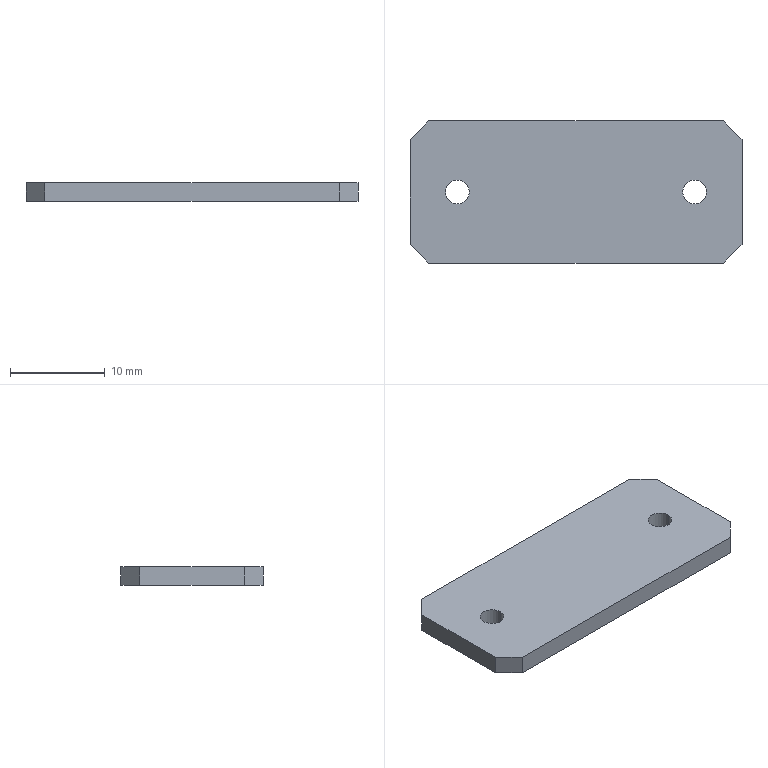Part | STEP file | 227H056374 Sensor Dog_Default | 1 solid | 14 faces | box 35 x 15 x 2 mm | volume 1014 mm3 | plane 10 | cylinder 4 | commonest cylinder face diameters 2.5 x4
STEP:
#1=CARTESIAN_POINT('',(0.,0.,0.));
#2=DIRECTION('',(0.,0.,1.));
#3=DIRECTION('',(1.,0.,0.));
#4=AXIS2_PLACEMENT_3D('',#1,#2,#3);
#5=CARTESIAN_POINT('',(-6.25,7.5,0.));
#6=VERTEX_POINT('',#5);
#7=CARTESIAN_POINT('',(-6.25,7.5,-2.));
#8=VERTEX_POINT('',#7);
#9=CARTESIAN_POINT('',(-6.25,7.5,-2.));
#10=DIRECTION('',(0.,0.,-1.));
#11=VECTOR('',#10,1.);
#12=LINE('',#9,#11);
#13=CARTESIAN_POINT('',(-5.,7.5,-2.));
#14=DIRECTION('',(0.,0.,-1.));
#15=DIRECTION('',(-1.,0.,0.));
#16=AXIS2_PLACEMENT_3D('',#13,#14,#15);
#17=CYLINDRICAL_SURFACE('',#16,1.25);
#18=CARTESIAN_POINT('',(6.283,0.));
#19=DIRECTION('',(0.,1.));
#20=VECTOR('',#19,1.);
#21=LINE('',#18,#20);
#22=(GEOMETRIC_REPRESENTATION_CONTEXT(2)PARAMETRIC_REPRESENTATION_CONTEXT()REPRESENTATION_CONTEXT('',''));
#23=DEFINITIONAL_REPRESENTATION('',(#21),#22);
#24=PCURVE('',#17,#23);
#25=CARTESIAN_POINT('',(-5.,7.5,-2.));
#26=DIRECTION('',(0.,0.,-1.));
#27=DIRECTION('',(-1.,0.,0.));
#28=AXIS2_PLACEMENT_3D('',#25,#26,#27);
#29=CYLINDRICAL_SURFACE('',#28,1.25);
#30=CARTESIAN_POINT('',(0.,0.));
#31=DIRECTION('',(0.,1.));
#32=VECTOR('',#31,1.);
#33=LINE('',#30,#32);
#34=(GEOMETRIC_REPRESENTATION_CONTEXT(2)PARAMETRIC_REPRESENTATION_CONTEXT()REPRESENTATION_CONTEXT('',''));
#35=DEFINITIONAL_REPRESENTATION('',(#33),#34);
#36=PCURVE('',#29,#35);
#37=SURFACE_CURVE('',#12,(#24,#36),.PCURVE_S1.);
#38=EDGE_CURVE('',#6,#8,#37,.T.);
#39=ORIENTED_EDGE('',*,*,#38,.T.);
#40=CARTESIAN_POINT('',(-3.75,7.5,-2.));
#41=VERTEX_POINT('',#40);
#42=CARTESIAN_POINT('',(-5.,7.5,-2.));
#43=DIRECTION('',(0.,0.,-1.));
#44=DIRECTION('',(-1.,0.,0.));
#45=AXIS2_PLACEMENT_3D('',#42,#43,#44);
#46=CIRCLE('',#45,1.25);
#47=CARTESIAN_POINT('',(0.,0.));
#48=DIRECTION('',(1.,0.));
#49=VECTOR('',#48,1.);
#50=LINE('',#47,#49);
#51=(GEOMETRIC_REPRESENTATION_CONTEXT(2)PARAMETRIC_REPRESENTATION_CONTEXT()REPRESENTATION_CONTEXT('',''));
#52=DEFINITIONAL_REPRESENTATION('',(#50),#51);
#53=PCURVE('',#17,#52);
#54=CARTESIAN_POINT('',(0.,15.,-2.));
#55=DIRECTION('',(0.,0.,1.));
#56=DIRECTION('',(1.,0.,0.));
#57=AXIS2_PLACEMENT_3D('',#54,#55,#56);
#58=PLANE('',#57);
#59=CARTESIAN_POINT('',(-6.25,-7.5));
#60=CARTESIAN_POINT('',(-6.25,-5.335));
#61=CARTESIAN_POINT('',(-4.375,-6.417));
#62=CARTESIAN_POINT('',(-2.5,-7.5));
#63=CARTESIAN_POINT('',(-4.375,-8.583));
#64=CARTESIAN_POINT('',(-6.25,-9.665));
#65=CARTESIAN_POINT('',(-6.25,-7.5));
#66=(BOUNDED_CURVE()B_SPLINE_CURVE(2,(#59,#60,#61,#62,#63,#64,#65),.UNSPECIFIED.,.T.,.F.)B_SPLINE_CURVE_WITH_KNOTS((1,2,2,2,2,1),(-2.094,0.,2.094,4.189,6.283,8.378),.UNSPECIFIED.)CURVE()GEOMETRIC_REPRESENTATION_ITEM()RATIONAL_B_SPLINE_CURVE((1.,0.5,1.,0.5,1.,0.5,1.))REPRESENTATION_ITEM(''));
#67=(GEOMETRIC_REPRESENTATION_CONTEXT(2)PARAMETRIC_REPRESENTATION_CONTEXT()REPRESENTATION_CONTEXT('',''));
#68=DEFINITIONAL_REPRESENTATION('',(#66),#67);
#69=PCURVE('',#58,#68);
#70=SURFACE_CURVE('',#46,(#53,#69),.PCURVE_S1.);
#71=EDGE_CURVE('',#41,#8,#70,.T.);
#72=ORIENTED_EDGE('',*,*,#71,.F.);
#73=CARTESIAN_POINT('',(-3.75,7.5,0.));
#74=VERTEX_POINT('',#73);
#75=CARTESIAN_POINT('',(-3.75,7.5,-2.));
#76=DIRECTION('',(0.,0.,-1.));
#77=VECTOR('',#76,1.);
#78=LINE('',#75,#77);
#79=CARTESIAN_POINT('',(3.142,0.));
#80=DIRECTION('',(0.,1.));
#81=VECTOR('',#80,1.);
#82=LINE('',#79,#81);
#83=(GEOMETRIC_REPRESENTATION_CONTEXT(2)PARAMETRIC_REPRESENTATION_CONTEXT()REPRESENTATION_CONTEXT('',''));
#84=DEFINITIONAL_REPRESENTATION('',(#82),#83);
#85=PCURVE('',#17,#84);
#86=CARTESIAN_POINT('',(3.142,0.));
#87=DIRECTION('',(0.,1.));
#88=VECTOR('',#87,1.);
#89=LINE('',#86,#88);
#90=(GEOMETRIC_REPRESENTATION_CONTEXT(2)PARAMETRIC_REPRESENTATION_CONTEXT()REPRESENTATION_CONTEXT('',''));
#91=DEFINITIONAL_REPRESENTATION('',(#89),#90);
#92=PCURVE('',#29,#91);
#93=SURFACE_CURVE('',#78,(#85,#92),.PCURVE_S1.);
#94=EDGE_CURVE('',#74,#41,#93,.T.);
#95=ORIENTED_EDGE('',*,*,#94,.F.);
#96=CARTESIAN_POINT('',(-5.,7.5,0.));
#97=DIRECTION('',(0.,0.,1.));
#98=DIRECTION('',(1.,0.,0.));
#99=AXIS2_PLACEMENT_3D('',#96,#97,#98);
#100=CIRCLE('',#99,1.25);
#101=CARTESIAN_POINT('',(9.425,-2.));
#102=DIRECTION('',(-1.,0.));
#103=VECTOR('',#102,1.);
#104=LINE('',#101,#103);
#105=(GEOMETRIC_REPRESENTATION_CONTEXT(2)PARAMETRIC_REPRESENTATION_CONTEXT()REPRESENTATION_CONTEXT('',''));
#106=DEFINITIONAL_REPRESENTATION('',(#104),#105);
#107=PCURVE('',#17,#106);
#108=CARTESIAN_POINT('',(0.,15.,0.));
#109=DIRECTION('',(0.,0.,1.));
#110=DIRECTION('',(1.,0.,0.));
#111=AXIS2_PLACEMENT_3D('',#108,#109,#110);
#112=PLANE('',#111);
#113=CARTESIAN_POINT('',(-5.,-7.5));
#114=DIRECTION('',(1.,0.));
#115=AXIS2_PLACEMENT_2D('',#113,#114);
#116=CIRCLE('',#115,1.25);
#117=(GEOMETRIC_REPRESENTATION_CONTEXT(2)PARAMETRIC_REPRESENTATION_CONTEXT()REPRESENTATION_CONTEXT('',''));
#118=DEFINITIONAL_REPRESENTATION('',(#116),#117);
#119=PCURVE('',#112,#118);
#120=SURFACE_CURVE('',#100,(#107,#119),.PCURVE_S1.);
#121=EDGE_CURVE('',#6,#74,#120,.T.);
#122=ORIENTED_EDGE('',*,*,#121,.F.);
#123=EDGE_LOOP('',(#39,#72,#95,#122));
#124=FACE_BOUND('',#123,.F.);
#125=ADVANCED_FACE('',(#124),#17,.F.);
#126=CARTESIAN_POINT('',(-31.25,7.5,0.));
#127=VERTEX_POINT('',#126);
#128=CARTESIAN_POINT('',(-31.25,7.5,-2.));
#129=VERTEX_POINT('',#128);
#130=CARTESIAN_POINT('',(-31.25,7.5,-2.));
#131=DIRECTION('',(0.,0.,-1.));
#132=VECTOR('',#131,1.);
#133=LINE('',#130,#132);
#134=CARTESIAN_POINT('',(-30.,7.5,-2.));
#135=DIRECTION('',(0.,0.,-1.));
#136=DIRECTION('',(-1.,0.,0.));
#137=AXIS2_PLACEMENT_3D('',#134,#135,#136);
#138=CYLINDRICAL_SURFACE('',#137,1.25);
#139=CARTESIAN_POINT('',(6.283,0.));
#140=DIRECTION('',(0.,1.));
#141=VECTOR('',#140,1.);
#142=LINE('',#139,#141);
#143=(GEOMETRIC_REPRESENTATION_CONTEXT(2)PARAMETRIC_REPRESENTATION_CONTEXT()REPRESENTATION_CONTEXT('',''));
#144=DEFINITIONAL_REPRESENTATION('',(#142),#143);
#145=PCURVE('',#138,#144);
#146=CARTESIAN_POINT('',(-30.,7.5,-2.));
#147=DIRECTION('',(0.,0.,-1.));
#148=DIRECTION('',(-1.,0.,0.));
#149=AXIS2_PLACEMENT_3D('',#146,#147,#148);
#150=CYLINDRICAL_SURFACE('',#149,1.25);
#151=CARTESIAN_POINT('',(0.,0.));
#152=DIRECTION('',(0.,1.));
#153=VECTOR('',#152,1.);
#154=LINE('',#151,#153);
#155=(GEOMETRIC_REPRESENTATION_CONTEXT(2)PARAMETRIC_REPRESENTATION_CONTEXT()REPRESENTATION_CONTEXT('',''));
#156=DEFINITIONAL_REPRESENTATION('',(#154),#155);
#157=PCURVE('',#150,#156);
#158=SURFACE_CURVE('',#133,(#145,#157),.PCURVE_S1.);
#159=EDGE_CURVE('',#127,#129,#158,.T.);
#160=ORIENTED_EDGE('',*,*,#159,.T.);
#161=CARTESIAN_POINT('',(-28.75,7.5,-2.));
#162=VERTEX_POINT('',#161);
#163=CARTESIAN_POINT('',(-30.,7.5,-2.));
#164=DIRECTION('',(0.,0.,-1.));
#165=DIRECTION('',(-1.,0.,0.));
#166=AXIS2_PLACEMENT_3D('',#163,#164,#165);
#167=CIRCLE('',#166,1.25);
#168=CARTESIAN_POINT('',(0.,0.));
#169=DIRECTION('',(1.,0.));
#170=VECTOR('',#169,1.);
#171=LINE('',#168,#170);
#172=(GEOMETRIC_REPRESENTATION_CONTEXT(2)PARAMETRIC_REPRESENTATION_CONTEXT()REPRESENTATION_CONTEXT('',''));
#173=DEFINITIONAL_REPRESENTATION('',(#171),#172);
#174=PCURVE('',#138,#173);
#175=CARTESIAN_POINT('',(-31.25,-7.5));
#176=CARTESIAN_POINT('',(-31.25,-5.335));
#177=CARTESIAN_POINT('',(-29.375,-6.417));
#178=CARTESIAN_POINT('',(-27.5,-7.5));
#179=CARTESIAN_POINT('',(-29.375,-8.583));
#180=CARTESIAN_POINT('',(-31.25,-9.665));
#181=CARTESIAN_POINT('',(-31.25,-7.5));
#182=(BOUNDED_CURVE()B_SPLINE_CURVE(2,(#175,#176,#177,#178,#179,#180,#181),.UNSPECIFIED.,.T.,.F.)B_SPLINE_CURVE_WITH_KNOTS((1,2,2,2,2,1),(-2.094,0.,2.094,4.189,6.283,8.378),.UNSPECIFIED.)CURVE()GEOMETRIC_REPRESENTATION_ITEM()RATIONAL_B_SPLINE_CURVE((1.,0.5,1.,0.5,1.,0.5,1.))REPRESENTATION_ITEM(''));
#183=(GEOMETRIC_REPRESENTATION_CONTEXT(2)PARAMETRIC_REPRESENTATION_CONTEXT()REPRESENTATION_CONTEXT('',''));
#184=DEFINITIONAL_REPRESENTATION('',(#182),#183);
#185=PCURVE('',#58,#184);
#186=SURFACE_CURVE('',#167,(#174,#185),.PCURVE_S1.);
#187=EDGE_CURVE('',#162,#129,#186,.T.);
#188=ORIENTED_EDGE('',*,*,#187,.F.);
#189=CARTESIAN_POINT('',(-28.75,7.5,0.));
#190=VERTEX_POINT('',#189);
#191=CARTESIAN_POINT('',(-28.75,7.5,-2.));
#192=DIRECTION('',(0.,0.,-1.));
#193=VECTOR('',#192,1.);
#194=LINE('',#191,#193);
#195=CARTESIAN_POINT('',(3.142,0.));
#196=DIRECTION('',(0.,1.));
#197=VECTOR('',#196,1.);
#198=LINE('',#195,#197);
#199=(GEOMETRIC_REPRESENTATION_CONTEXT(2)PARAMETRIC_REPRESENTATION_CONTEXT()REPRESENTATION_CONTEXT('',''));
#200=DEFINITIONAL_REPRESENTATION('',(#198),#199);
#201=PCURVE('',#138,#200);
#202=CARTESIAN_POINT('',(3.142,0.));
#203=DIRECTION('',(0.,1.));
#204=VECTOR('',#203,1.);
#205=LINE('',#202,#204);
#206=(GEOMETRIC_REPRESENTATION_CONTEXT(2)PARAMETRIC_REPRESENTATION_CONTEXT()REPRESENTATION_CONTEXT('',''));
#207=DEFINITIONAL_REPRESENTATION('',(#205),#206);
#208=PCURVE('',#150,#207);
#209=SURFACE_CURVE('',#194,(#201,#208),.PCURVE_S1.);
#210=EDGE_CURVE('',#190,#162,#209,.T.);
#211=ORIENTED_EDGE('',*,*,#210,.F.);
#212=CARTESIAN_POINT('',(-30.,7.5,0.));
#213=DIRECTION('',(0.,0.,1.));
#214=DIRECTION('',(1.,0.,0.));
#215=AXIS2_PLACEMENT_3D('',#212,#213,#214);
#216=CIRCLE('',#215,1.25);
#217=CARTESIAN_POINT('',(9.425,-2.));
#218=DIRECTION('',(-1.,0.));
#219=VECTOR('',#218,1.);
#220=LINE('',#217,#219);
#221=(GEOMETRIC_REPRESENTATION_CONTEXT(2)PARAMETRIC_REPRESENTATION_CONTEXT()REPRESENTATION_CONTEXT('',''));
#222=DEFINITIONAL_REPRESENTATION('',(#220),#221);
#223=PCURVE('',#138,#222);
#224=CARTESIAN_POINT('',(-30.,-7.5));
#225=DIRECTION('',(1.,0.));
#226=AXIS2_PLACEMENT_2D('',#224,#225);
#227=CIRCLE('',#226,1.25);
#228=(GEOMETRIC_REPRESENTATION_CONTEXT(2)PARAMETRIC_REPRESENTATION_CONTEXT()REPRESENTATION_CONTEXT('',''));
#229=DEFINITIONAL_REPRESENTATION('',(#227),#228);
#230=PCURVE('',#112,#229);
#231=SURFACE_CURVE('',#216,(#223,#230),.PCURVE_S1.);
#232=EDGE_CURVE('',#127,#190,#231,.T.);
#233=ORIENTED_EDGE('',*,*,#232,.F.);
#234=EDGE_LOOP('',(#160,#188,#211,#233));
#235=FACE_BOUND('',#234,.F.);
#236=ADVANCED_FACE('',(#235),#138,.F.);
#237=CARTESIAN_POINT('',(-5.,7.5,-2.));
#238=DIRECTION('',(0.,0.,-1.));
#239=DIRECTION('',(-1.,0.,0.));
#240=AXIS2_PLACEMENT_3D('',#237,#238,#239);
#241=CIRCLE('',#240,1.25);
#242=CARTESIAN_POINT('',(-6.25,-7.5));
#243=CARTESIAN_POINT('',(-6.25,-5.335));
#244=CARTESIAN_POINT('',(-4.375,-6.417));
#245=CARTESIAN_POINT('',(-2.5,-7.5));
#246=CARTESIAN_POINT('',(-4.375,-8.583));
#247=CARTESIAN_POINT('',(-6.25,-9.665));
#248=CARTESIAN_POINT('',(-6.25,-7.5));
#249=(BOUNDED_CURVE()B_SPLINE_CURVE(2,(#242,#243,#244,#245,#246,#247,#248),.UNSPECIFIED.,.T.,.F.)B_SPLINE_CURVE_WITH_KNOTS((1,2,2,2,2,1),(-2.094,0.,2.094,4.189,6.283,8.378),.UNSPECIFIED.)CURVE()GEOMETRIC_REPRESENTATION_ITEM()RATIONAL_B_SPLINE_CURVE((1.,0.5,1.,0.5,1.,0.5,1.))REPRESENTATION_ITEM(''));
#250=(GEOMETRIC_REPRESENTATION_CONTEXT(2)PARAMETRIC_REPRESENTATION_CONTEXT()REPRESENTATION_CONTEXT('',''));
#251=DEFINITIONAL_REPRESENTATION('',(#249),#250);
#252=PCURVE('',#58,#251);
#253=CARTESIAN_POINT('',(0.,0.));
#254=DIRECTION('',(1.,0.));
#255=VECTOR('',#254,1.);
#256=LINE('',#253,#255);
#257=(GEOMETRIC_REPRESENTATION_CONTEXT(2)PARAMETRIC_REPRESENTATION_CONTEXT()REPRESENTATION_CONTEXT('',''));
#258=DEFINITIONAL_REPRESENTATION('',(#256),#257);
#259=PCURVE('',#29,#258);
#260=SURFACE_CURVE('',#241,(#252,#259),.PCURVE_S1.);
#261=EDGE_CURVE('',#8,#41,#260,.T.);
#262=ORIENTED_EDGE('',*,*,#261,.F.);
#263=ORIENTED_EDGE('',*,*,#71,.F.);
#264=EDGE_LOOP('',(#262,#263));
#265=FACE_BOUND('',#264,.T.);
#266=CARTESIAN_POINT('',(-30.,7.5,-2.));
#267=DIRECTION('',(0.,0.,-1.));
#268=DIRECTION('',(-1.,0.,0.));
#269=AXIS2_PLACEMENT_3D('',#266,#267,#268);
#270=CIRCLE('',#269,1.25);
#271=CARTESIAN_POINT('',(-31.25,-7.5));
#272=CARTESIAN_POINT('',(-31.25,-5.335));
#273=CARTESIAN_POINT('',(-29.375,-6.417));
#274=CARTESIAN_POINT('',(-27.5,-7.5));
#275=CARTESIAN_POINT('',(-29.375,-8.583));
#276=CARTESIAN_POINT('',(-31.25,-9.665));
#277=CARTESIAN_POINT('',(-31.25,-7.5));
#278=(BOUNDED_CURVE()B_SPLINE_CURVE(2,(#271,#272,#273,#274,#275,#276,#277),.UNSPECIFIED.,.T.,.F.)B_SPLINE_CURVE_WITH_KNOTS((1,2,2,2,2,1),(-2.094,0.,2.094,4.189,6.283,8.378),.UNSPECIFIED.)CURVE()GEOMETRIC_REPRESENTATION_ITEM()RATIONAL_B_SPLINE_CURVE((1.,0.5,1.,0.5,1.,0.5,1.))REPRESENTATION_ITEM(''));
#279=(GEOMETRIC_REPRESENTATION_CONTEXT(2)PARAMETRIC_REPRESENTATION_CONTEXT()REPRESENTATION_CONTEXT('',''));
#280=DEFINITIONAL_REPRESENTATION('',(#278),#279);
#281=PCURVE('',#58,#280);
#282=CARTESIAN_POINT('',(0.,0.));
#283=DIRECTION('',(1.,0.));
#284=VECTOR('',#283,1.);
#285=LINE('',#282,#284);
#286=(GEOMETRIC_REPRESENTATION_CONTEXT(2)PARAMETRIC_REPRESENTATION_CONTEXT()REPRESENTATION_CONTEXT('',''));
#287=DEFINITIONAL_REPRESENTATION('',(#285),#286);
#288=PCURVE('',#150,#287);
#289=SURFACE_CURVE('',#270,(#281,#288),.PCURVE_S1.);
#290=EDGE_CURVE('',#129,#162,#289,.T.);
#291=ORIENTED_EDGE('',*,*,#290,.F.);
#292=ORIENTED_EDGE('',*,*,#187,.F.);
#293=EDGE_LOOP('',(#291,#292));
#294=FACE_BOUND('',#293,.T.);
#295=CARTESIAN_POINT('',(-2.,0.,-2.));
#296=VERTEX_POINT('',#295);
#297=CARTESIAN_POINT('',(-33.,0.,-2.));
#298=VERTEX_POINT('',#297);
#299=CARTESIAN_POINT('',(0.,0.,-2.));
#300=DIRECTION('',(-1.,0.,0.));
#301=VECTOR('',#300,1.);
#302=LINE('',#299,#301);
#303=CARTESIAN_POINT('',(0.,-15.));
#304=DIRECTION('',(-1.,0.));
#305=VECTOR('',#304,1.);
#306=LINE('',#303,#305);
#307=(GEOMETRIC_REPRESENTATION_CONTEXT(2)PARAMETRIC_REPRESENTATION_CONTEXT()REPRESENTATION_CONTEXT('',''));
#308=DEFINITIONAL_REPRESENTATION('',(#306),#307);
#309=PCURVE('',#58,#308);
#310=CARTESIAN_POINT('',(0.,0.,0.));
#311=DIRECTION('',(0.,1.,0.));
#312=DIRECTION('',(1.,0.,0.));
#313=AXIS2_PLACEMENT_3D('',#310,#311,#312);
#314=PLANE('',#313);
#315=CARTESIAN_POINT('',(0.,2.));
#316=DIRECTION('',(-1.,0.));
#317=VECTOR('',#316,1.);
#318=LINE('',#315,#317);
#319=(GEOMETRIC_REPRESENTATION_CONTEXT(2)PARAMETRIC_REPRESENTATION_CONTEXT()REPRESENTATION_CONTEXT('',''));
#320=DEFINITIONAL_REPRESENTATION('',(#318),#319);
#321=PCURVE('',#314,#320);
#322=SURFACE_CURVE('',#302,(#309,#321),.PCURVE_S1.);
#323=EDGE_CURVE('',#296,#298,#322,.T.);
#324=ORIENTED_EDGE('',*,*,#323,.T.);
#325=CARTESIAN_POINT('',(-35.,2.,-2.));
#326=VERTEX_POINT('',#325);
#327=CARTESIAN_POINT('',(-33.,0.,-2.));
#328=DIRECTION('',(-0.7071,0.7071,0.));
#329=VECTOR('',#328,1.);
#330=LINE('',#327,#329);
#331=CARTESIAN_POINT('',(-33.,-15.));
#332=DIRECTION('',(-0.7071,0.7071));
#333=VECTOR('',#332,1.);
#334=LINE('',#331,#333);
#335=(GEOMETRIC_REPRESENTATION_CONTEXT(2)PARAMETRIC_REPRESENTATION_CONTEXT()REPRESENTATION_CONTEXT('',''));
#336=DEFINITIONAL_REPRESENTATION('',(#334),#335);
#337=PCURVE('',#58,#336);
#338=CARTESIAN_POINT('',(-33.,0.,0.));
#339=DIRECTION('',(-0.7071,-0.7071,0.));
#340=DIRECTION('',(0.,0.,1.));
#341=AXIS2_PLACEMENT_3D('',#338,#339,#340);
#342=PLANE('',#341);
#343=CARTESIAN_POINT('',(-2.,0.));
#344=DIRECTION('',(0.,1.));
#345=VECTOR('',#344,1.);
#346=LINE('',#343,#345);
#347=(GEOMETRIC_REPRESENTATION_CONTEXT(2)PARAMETRIC_REPRESENTATION_CONTEXT()REPRESENTATION_CONTEXT('',''));
#348=DEFINITIONAL_REPRESENTATION('',(#346),#347);
#349=PCURVE('',#342,#348);
#350=SURFACE_CURVE('',#330,(#337,#349),.PCURVE_S1.);
#351=EDGE_CURVE('',#298,#326,#350,.T.);
#352=ORIENTED_EDGE('',*,*,#351,.T.);
#353=CARTESIAN_POINT('',(-35.,13.,-2.));
#354=VERTEX_POINT('',#353);
#355=CARTESIAN_POINT('',(-35.,15.,-2.));
#356=DIRECTION('',(0.,-1.,0.));
#357=VECTOR('',#356,1.);
#358=LINE('',#355,#357);
#359=CARTESIAN_POINT('',(-35.,0.));
#360=DIRECTION('',(0.,-1.));
#361=VECTOR('',#360,1.);
#362=LINE('',#359,#361);
#363=(GEOMETRIC_REPRESENTATION_CONTEXT(2)PARAMETRIC_REPRESENTATION_CONTEXT()REPRESENTATION_CONTEXT('',''));
#364=DEFINITIONAL_REPRESENTATION('',(#362),#363);
#365=PCURVE('',#58,#364);
#366=CARTESIAN_POINT('',(-35.,15.,0.));
#367=DIRECTION('',(-1.,0.,0.));
#368=DIRECTION('',(0.,0.,1.));
#369=AXIS2_PLACEMENT_3D('',#366,#367,#368);
#370=PLANE('',#369);
#371=CARTESIAN_POINT('',(-2.,0.));
#372=DIRECTION('',(0.,-1.));
#373=VECTOR('',#372,1.);
#374=LINE('',#371,#373);
#375=(GEOMETRIC_REPRESENTATION_CONTEXT(2)PARAMETRIC_REPRESENTATION_CONTEXT()REPRESENTATION_CONTEXT('',''));
#376=DEFINITIONAL_REPRESENTATION('',(#374),#375);
#377=PCURVE('',#370,#376);
#378=SURFACE_CURVE('',#358,(#365,#377),.PCURVE_S1.);
#379=EDGE_CURVE('',#354,#326,#378,.T.);
#380=ORIENTED_EDGE('',*,*,#379,.F.);
#381=CARTESIAN_POINT('',(-33.,15.,-2.));
#382=VERTEX_POINT('',#381);
#383=CARTESIAN_POINT('',(-35.,13.,-2.));
#384=DIRECTION('',(0.7071,0.7071,0.));
#385=VECTOR('',#384,1.);
#386=LINE('',#383,#385);
#387=CARTESIAN_POINT('',(-35.,-2.));
#388=DIRECTION('',(0.7071,0.7071));
#389=VECTOR('',#388,1.);
#390=LINE('',#387,#389);
#391=(GEOMETRIC_REPRESENTATION_CONTEXT(2)PARAMETRIC_REPRESENTATION_CONTEXT()REPRESENTATION_CONTEXT('',''));
#392=DEFINITIONAL_REPRESENTATION('',(#390),#391);
#393=PCURVE('',#58,#392);
#394=CARTESIAN_POINT('',(-35.,13.,0.));
#395=DIRECTION('',(0.7071,-0.7071,0.));
#396=DIRECTION('',(0.,0.,-1.));
#397=AXIS2_PLACEMENT_3D('',#394,#395,#396);
#398=PLANE('',#397);
#399=CARTESIAN_POINT('',(2.,0.));
#400=DIRECTION('',(0.,1.));
#401=VECTOR('',#400,1.);
#402=LINE('',#399,#401);
#403=(GEOMETRIC_REPRESENTATION_CONTEXT(2)PARAMETRIC_REPRESENTATION_CONTEXT()REPRESENTATION_CONTEXT('',''));
#404=DEFINITIONAL_REPRESENTATION('',(#402),#403);
#405=PCURVE('',#398,#404);
#406=SURFACE_CURVE('',#386,(#393,#405),.PCURVE_S1.);
#407=EDGE_CURVE('',#354,#382,#406,.T.);
#408=ORIENTED_EDGE('',*,*,#407,.T.);
#409=CARTESIAN_POINT('',(-2.,15.,-2.));
#410=VERTEX_POINT('',#409);
#411=CARTESIAN_POINT('',(0.,15.,-2.));
#412=DIRECTION('',(-1.,0.,0.));
#413=VECTOR('',#412,1.);
#414=LINE('',#411,#413);
#415=CARTESIAN_POINT('',(0.,0.));
#416=DIRECTION('',(-1.,0.));
#417=VECTOR('',#416,1.);
#418=LINE('',#415,#417);
#419=(GEOMETRIC_REPRESENTATION_CONTEXT(2)PARAMETRIC_REPRESENTATION_CONTEXT()REPRESENTATION_CONTEXT('',''));
#420=DEFINITIONAL_REPRESENTATION('',(#418),#419);
#421=PCURVE('',#58,#420);
#422=CARTESIAN_POINT('',(0.,15.,0.));
#423=DIRECTION('',(0.,1.,0.));
#424=DIRECTION('',(1.,0.,0.));
#425=AXIS2_PLACEMENT_3D('',#422,#423,#424);
#426=PLANE('',#425);
#427=CARTESIAN_POINT('',(0.,2.));
#428=DIRECTION('',(-1.,0.));
#429=VECTOR('',#428,1.);
#430=LINE('',#427,#429);
#431=(GEOMETRIC_REPRESENTATION_CONTEXT(2)PARAMETRIC_REPRESENTATION_CONTEXT()REPRESENTATION_CONTEXT('',''));
#432=DEFINITIONAL_REPRESENTATION('',(#430),#431);
#433=PCURVE('',#426,#432);
#434=SURFACE_CURVE('',#414,(#421,#433),.PCURVE_S1.);
#435=EDGE_CURVE('',#410,#382,#434,.T.);
#436=ORIENTED_EDGE('',*,*,#435,.F.);
#437=CARTESIAN_POINT('',(0.,13.,-2.));
#438=VERTEX_POINT('',#437);
#439=CARTESIAN_POINT('',(0.,13.,-2.));
#440=DIRECTION('',(0.7071,-0.7071,0.));
#441=VECTOR('',#440,1.);
#442=LINE('',#439,#441);
#443=CARTESIAN_POINT('',(0.,-2.));
#444=DIRECTION('',(0.7071,-0.7071));
#445=VECTOR('',#444,1.);
#446=LINE('',#443,#445);
#447=(GEOMETRIC_REPRESENTATION_CONTEXT(2)PARAMETRIC_REPRESENTATION_CONTEXT()REPRESENTATION_CONTEXT('',''));
#448=DEFINITIONAL_REPRESENTATION('',(#446),#447);
#449=PCURVE('',#58,#448);
#450=CARTESIAN_POINT('',(0.,13.,-2.));
#451=DIRECTION('',(-0.7071,-0.7071,0.));
#452=DIRECTION('',(0.,0.,1.));
#453=AXIS2_PLACEMENT_3D('',#450,#451,#452);
#454=PLANE('',#453);
#455=CARTESIAN_POINT('',(0.,0.));
#456=DIRECTION('',(0.,-1.));
#457=VECTOR('',#456,1.);
#458=LINE('',#455,#457);
#459=(GEOMETRIC_REPRESENTATION_CONTEXT(2)PARAMETRIC_REPRESENTATION_CONTEXT()REPRESENTATION_CONTEXT('',''));
#460=DEFINITIONAL_REPRESENTATION('',(#458),#459);
#461=PCURVE('',#454,#460);
#462=SURFACE_CURVE('',#442,(#449,#461),.PCURVE_S1.);
#463=EDGE_CURVE('',#410,#438,#462,.T.);
#464=ORIENTED_EDGE('',*,*,#463,.T.);
#465=CARTESIAN_POINT('',(0.,2.,-2.));
#466=VERTEX_POINT('',#465);
#467=CARTESIAN_POINT('',(0.,15.,-2.));
#468=DIRECTION('',(0.,-1.,0.));
#469=VECTOR('',#468,1.);
#470=LINE('',#467,#469);
#471=CARTESIAN_POINT('',(0.,0.));
#472=DIRECTION('',(0.,-1.));
#473=VECTOR('',#472,1.);
#474=LINE('',#471,#473);
#475=(GEOMETRIC_REPRESENTATION_CONTEXT(2)PARAMETRIC_REPRESENTATION_CONTEXT()REPRESENTATION_CONTEXT('',''));
#476=DEFINITIONAL_REPRESENTATION('',(#474),#475);
#477=PCURVE('',#58,#476);
#478=CARTESIAN_POINT('',(0.,15.,-2.));
#479=DIRECTION('',(1.,0.,0.));
#480=DIRECTION('',(0.,0.,-1.));
#481=AXIS2_PLACEMENT_3D('',#478,#479,#480);
#482=PLANE('',#481);
#483=CARTESIAN_POINT('',(0.,0.));
#484=DIRECTION('',(0.,-1.));
#485=VECTOR('',#484,1.);
#486=LINE('',#483,#485);
#487=(GEOMETRIC_REPRESENTATION_CONTEXT(2)PARAMETRIC_REPRESENTATION_CONTEXT()REPRESENTATION_CONTEXT('',''));
#488=DEFINITIONAL_REPRESENTATION('',(#486),#487);
#489=PCURVE('',#482,#488);
#490=SURFACE_CURVE('',#470,(#477,#489),.PCURVE_S1.);
#491=EDGE_CURVE('',#438,#466,#490,.T.);
#492=ORIENTED_EDGE('',*,*,#491,.T.);
#493=CARTESIAN_POINT('',(-2.,0.,-2.));
#494=DIRECTION('',(-0.7071,-0.7071,0.));
#495=VECTOR('',#494,1.);
#496=LINE('',#493,#495);
#497=CARTESIAN_POINT('',(-2.,-15.));
#498=DIRECTION('',(-0.7071,-0.7071));
#499=VECTOR('',#498,1.);
#500=LINE('',#497,#499);
#501=(GEOMETRIC_REPRESENTATION_CONTEXT(2)PARAMETRIC_REPRESENTATION_CONTEXT()REPRESENTATION_CONTEXT('',''));
#502=DEFINITIONAL_REPRESENTATION('',(#500),#501);
#503=PCURVE('',#58,#502);
#504=CARTESIAN_POINT('',(-2.,0.,0.));
#505=DIRECTION('',(0.7071,-0.7071,0.));
#506=DIRECTION('',(0.,0.,-1.));
#507=AXIS2_PLACEMENT_3D('',#504,#505,#506);
#508=PLANE('',#507);
#509=CARTESIAN_POINT('',(2.,0.));
#510=DIRECTION('',(0.,-1.));
#511=VECTOR('',#510,1.);
#512=LINE('',#509,#511);
#513=(GEOMETRIC_REPRESENTATION_CONTEXT(2)PARAMETRIC_REPRESENTATION_CONTEXT()REPRESENTATION_CONTEXT('',''));
#514=DEFINITIONAL_REPRESENTATION('',(#512),#513);
#515=PCURVE('',#508,#514);
#516=SURFACE_CURVE('',#496,(#503,#515),.PCURVE_S1.);
#517=EDGE_CURVE('',#466,#296,#516,.T.);
#518=ORIENTED_EDGE('',*,*,#517,.T.);
#519=EDGE_LOOP('',(#324,#352,#380,#408,#436,#464,#492,#518));
#520=FACE_BOUND('',#519,.T.);
#521=ADVANCED_FACE('',(#265,#294,#520),#58,.F.);
#522=ORIENTED_EDGE('',*,*,#379,.T.);
#523=CARTESIAN_POINT('',(-35.,2.,0.));
#524=VERTEX_POINT('',#523);
#525=CARTESIAN_POINT('',(-35.,2.,0.));
#526=DIRECTION('',(0.,0.,1.));
#527=VECTOR('',#526,1.);
#528=LINE('',#525,#527);
#529=CARTESIAN_POINT('',(0.,-13.));
#530=DIRECTION('',(1.,0.));
#531=VECTOR('',#530,1.);
#532=LINE('',#529,#531);
#533=(GEOMETRIC_REPRESENTATION_CONTEXT(2)PARAMETRIC_REPRESENTATION_CONTEXT()REPRESENTATION_CONTEXT('',''));
#534=DEFINITIONAL_REPRESENTATION('',(#532),#533);
#535=PCURVE('',#370,#534);
#536=CARTESIAN_POINT('',(0.,2.828));
#537=DIRECTION('',(1.,0.));
#538=VECTOR('',#537,1.);
#539=LINE('',#536,#538);
#540=(GEOMETRIC_REPRESENTATION_CONTEXT(2)PARAMETRIC_REPRESENTATION_CONTEXT()REPRESENTATION_CONTEXT('',''));
#541=DEFINITIONAL_REPRESENTATION('',(#539),#540);
#542=PCURVE('',#342,#541);
#543=SURFACE_CURVE('',#528,(#535,#542),.PCURVE_S1.);
#544=EDGE_CURVE('',#326,#524,#543,.T.);
#545=ORIENTED_EDGE('',*,*,#544,.T.);
#546=CARTESIAN_POINT('',(-35.,13.,0.));
#547=VERTEX_POINT('',#546);
#548=CARTESIAN_POINT('',(-35.,15.,0.));
#549=DIRECTION('',(0.,-1.,0.));
#550=VECTOR('',#549,1.);
#551=LINE('',#548,#550);
#552=CARTESIAN_POINT('',(0.,0.));
#553=DIRECTION('',(0.,-1.));
#554=VECTOR('',#553,1.);
#555=LINE('',#552,#554);
#556=(GEOMETRIC_REPRESENTATION_CONTEXT(2)PARAMETRIC_REPRESENTATION_CONTEXT()REPRESENTATION_CONTEXT('',''));
#557=DEFINITIONAL_REPRESENTATION('',(#555),#556);
#558=PCURVE('',#370,#557);
#559=CARTESIAN_POINT('',(-35.,0.));
#560=DIRECTION('',(0.,-1.));
#561=VECTOR('',#560,1.);
#562=LINE('',#559,#561);
#563=(GEOMETRIC_REPRESENTATION_CONTEXT(2)PARAMETRIC_REPRESENTATION_CONTEXT()REPRESENTATION_CONTEXT('',''));
#564=DEFINITIONAL_REPRESENTATION('',(#562),#563);
#565=PCURVE('',#112,#564);
#566=SURFACE_CURVE('',#551,(#558,#565),.PCURVE_S1.);
#567=EDGE_CURVE('',#547,#524,#566,.T.);
#568=ORIENTED_EDGE('',*,*,#567,.F.);
#569=CARTESIAN_POINT('',(-35.,13.,0.));
#570=DIRECTION('',(0.,0.,-1.));
#571=VECTOR('',#570,1.);
#572=LINE('',#569,#571);
#573=CARTESIAN_POINT('',(0.,-2.));
#574=DIRECTION('',(-1.,0.));
#575=VECTOR('',#574,1.);
#576=LINE('',#573,#575);
#577=(GEOMETRIC_REPRESENTATION_CONTEXT(2)PARAMETRIC_REPRESENTATION_CONTEXT()REPRESENTATION_CONTEXT('',''));
#578=DEFINITIONAL_REPRESENTATION('',(#576),#577);
#579=PCURVE('',#370,#578);
#580=CARTESIAN_POINT('',(0.,0.));
#581=DIRECTION('',(1.,0.));
#582=VECTOR('',#581,1.);
#583=LINE('',#580,#582);
#584=(GEOMETRIC_REPRESENTATION_CONTEXT(2)PARAMETRIC_REPRESENTATION_CONTEXT()REPRESENTATION_CONTEXT('',''));
#585=DEFINITIONAL_REPRESENTATION('',(#583),#584);
#586=PCURVE('',#398,#585);
#587=SURFACE_CURVE('',#572,(#579,#586),.PCURVE_S1.);
#588=EDGE_CURVE('',#547,#354,#587,.T.);
#589=ORIENTED_EDGE('',*,*,#588,.T.);
#590=EDGE_LOOP('',(#522,#545,#568,#589));
#591=FACE_BOUND('',#590,.T.);
#592=ADVANCED_FACE('',(#591),#370,.T.);
#593=ORIENTED_EDGE('',*,*,#121,.F.);
#594=CARTESIAN_POINT('',(-5.,7.5,0.));
#595=DIRECTION('',(0.,0.,1.));
#596=DIRECTION('',(1.,0.,0.));
#597=AXIS2_PLACEMENT_3D('',#594,#595,#596);
#598=CIRCLE('',#597,1.25);
#599=CARTESIAN_POINT('',(-5.,-7.5));
#600=DIRECTION('',(1.,0.));
#601=AXIS2_PLACEMENT_2D('',#599,#600);
#602=CIRCLE('',#601,1.25);
#603=(GEOMETRIC_REPRESENTATION_CONTEXT(2)PARAMETRIC_REPRESENTATION_CONTEXT()REPRESENTATION_CONTEXT('',''));
#604=DEFINITIONAL_REPRESENTATION('',(#602),#603);
#605=PCURVE('',#112,#604);
#606=CARTESIAN_POINT('',(3.142,-2.));
#607=DIRECTION('',(-1.,0.));
#608=VECTOR('',#607,1.);
#609=LINE('',#606,#608);
#610=(GEOMETRIC_REPRESENTATION_CONTEXT(2)PARAMETRIC_REPRESENTATION_CONTEXT()REPRESENTATION_CONTEXT('',''));
#611=DEFINITIONAL_REPRESENTATION('',(#609),#610);
#612=PCURVE('',#29,#611);
#613=SURFACE_CURVE('',#598,(#605,#612),.PCURVE_S1.);
#614=EDGE_CURVE('',#74,#6,#613,.T.);
#615=ORIENTED_EDGE('',*,*,#614,.F.);
#616=EDGE_LOOP('',(#593,#615));
#617=FACE_BOUND('',#616,.T.);
#618=ORIENTED_EDGE('',*,*,#232,.F.);
#619=CARTESIAN_POINT('',(-30.,7.5,0.));
#620=DIRECTION('',(0.,0.,1.));
#621=DIRECTION('',(1.,0.,0.));
#622=AXIS2_PLACEMENT_3D('',#619,#620,#621);
#623=CIRCLE('',#622,1.25);
#624=CARTESIAN_POINT('',(-30.,-7.5));
#625=DIRECTION('',(1.,0.));
#626=AXIS2_PLACEMENT_2D('',#624,#625);
#627=CIRCLE('',#626,1.25);
#628=(GEOMETRIC_REPRESENTATION_CONTEXT(2)PARAMETRIC_REPRESENTATION_CONTEXT()REPRESENTATION_CONTEXT('',''));
#629=DEFINITIONAL_REPRESENTATION('',(#627),#628);
#630=PCURVE('',#112,#629);
#631=CARTESIAN_POINT('',(3.142,-2.));
#632=DIRECTION('',(-1.,0.));
#633=VECTOR('',#632,1.);
#634=LINE('',#631,#633);
#635=(GEOMETRIC_REPRESENTATION_CONTEXT(2)PARAMETRIC_REPRESENTATION_CONTEXT()REPRESENTATION_CONTEXT('',''));
#636=DEFINITIONAL_REPRESENTATION('',(#634),#635);
#637=PCURVE('',#150,#636);
#638=SURFACE_CURVE('',#623,(#630,#637),.PCURVE_S1.);
#639=EDGE_CURVE('',#190,#127,#638,.T.);
#640=ORIENTED_EDGE('',*,*,#639,.F.);
#641=EDGE_LOOP('',(#618,#640));
#642=FACE_BOUND('',#641,.T.);
#643=ORIENTED_EDGE('',*,*,#567,.T.);
#644=CARTESIAN_POINT('',(-33.,0.,0.));
#645=VERTEX_POINT('',#644);
#646=CARTESIAN_POINT('',(-24.,-9.,0.));
#647=DIRECTION('',(0.7071,-0.7071,0.));
#648=VECTOR('',#647,1.);
#649=LINE('',#646,#648);
#650=CARTESIAN_POINT('',(-24.,-24.));
#651=DIRECTION('',(0.7071,-0.7071));
#652=VECTOR('',#651,1.);
#653=LINE('',#650,#652);
#654=(GEOMETRIC_REPRESENTATION_CONTEXT(2)PARAMETRIC_REPRESENTATION_CONTEXT()REPRESENTATION_CONTEXT('',''));
#655=DEFINITIONAL_REPRESENTATION('',(#653),#654);
#656=PCURVE('',#112,#655);
#657=CARTESIAN_POINT('',(0.,-12.728));
#658=DIRECTION('',(0.,-1.));
#659=VECTOR('',#658,1.);
#660=LINE('',#657,#659);
#661=(GEOMETRIC_REPRESENTATION_CONTEXT(2)PARAMETRIC_REPRESENTATION_CONTEXT()REPRESENTATION_CONTEXT('',''));
#662=DEFINITIONAL_REPRESENTATION('',(#660),#661);
#663=PCURVE('',#342,#662);
#664=SURFACE_CURVE('',#649,(#656,#663),.PCURVE_S1.);
#665=EDGE_CURVE('',#524,#645,#664,.T.);
#666=ORIENTED_EDGE('',*,*,#665,.T.);
#667=CARTESIAN_POINT('',(-2.,0.,0.));
#668=VERTEX_POINT('',#667);
#669=CARTESIAN_POINT('',(0.,0.,0.));
#670=DIRECTION('',(-1.,0.,0.));
#671=VECTOR('',#670,1.);
#672=LINE('',#669,#671);
#673=CARTESIAN_POINT('',(0.,-15.));
#674=DIRECTION('',(-1.,0.));
#675=VECTOR('',#674,1.);
#676=LINE('',#673,#675);
#677=(GEOMETRIC_REPRESENTATION_CONTEXT(2)PARAMETRIC_REPRESENTATION_CONTEXT()REPRESENTATION_CONTEXT('',''));
#678=DEFINITIONAL_REPRESENTATION('',(#676),#677);
#679=PCURVE('',#112,#678);
#680=CARTESIAN_POINT('',(0.,0.));
#681=DIRECTION('',(-1.,0.));
#682=VECTOR('',#681,1.);
#683=LINE('',#680,#682);
#684=(GEOMETRIC_REPRESENTATION_CONTEXT(2)PARAMETRIC_REPRESENTATION_CONTEXT()REPRESENTATION_CONTEXT('',''));
#685=DEFINITIONAL_REPRESENTATION('',(#683),#684);
#686=PCURVE('',#314,#685);
#687=SURFACE_CURVE('',#672,(#679,#686),.PCURVE_S1.);
#688=EDGE_CURVE('',#668,#645,#687,.T.);
#689=ORIENTED_EDGE('',*,*,#688,.F.);
#690=CARTESIAN_POINT('',(0.,2.,0.));
#691=VERTEX_POINT('',#690);
#692=CARTESIAN_POINT('',(6.5,8.5,0.));
#693=DIRECTION('',(0.7071,0.7071,0.));
#694=VECTOR('',#693,1.);
#695=LINE('',#692,#694);
#696=CARTESIAN_POINT('',(6.5,-6.5));
#697=DIRECTION('',(0.7071,0.7071));
#698=VECTOR('',#697,1.);
#699=LINE('',#696,#698);
#700=(GEOMETRIC_REPRESENTATION_CONTEXT(2)PARAMETRIC_REPRESENTATION_CONTEXT()REPRESENTATION_CONTEXT('',''));
#701=DEFINITIONAL_REPRESENTATION('',(#699),#700);
#702=PCURVE('',#112,#701);
#703=CARTESIAN_POINT('',(0.,12.021));
#704=DIRECTION('',(0.,1.));
#705=VECTOR('',#704,1.);
#706=LINE('',#703,#705);
#707=(GEOMETRIC_REPRESENTATION_CONTEXT(2)PARAMETRIC_REPRESENTATION_CONTEXT()REPRESENTATION_CONTEXT('',''));
#708=DEFINITIONAL_REPRESENTATION('',(#706),#707);
#709=PCURVE('',#508,#708);
#710=SURFACE_CURVE('',#695,(#702,#709),.PCURVE_S1.);
#711=EDGE_CURVE('',#668,#691,#710,.T.);
#712=ORIENTED_EDGE('',*,*,#711,.T.);
#713=CARTESIAN_POINT('',(0.,13.,0.));
#714=VERTEX_POINT('',#713);
#715=CARTESIAN_POINT('',(0.,15.,0.));
#716=DIRECTION('',(0.,-1.,0.));
#717=VECTOR('',#716,1.);
#718=LINE('',#715,#717);
#719=CARTESIAN_POINT('',(0.,0.));
#720=DIRECTION('',(0.,-1.));
#721=VECTOR('',#720,1.);
#722=LINE('',#719,#721);
#723=(GEOMETRIC_REPRESENTATION_CONTEXT(2)PARAMETRIC_REPRESENTATION_CONTEXT()REPRESENTATION_CONTEXT('',''));
#724=DEFINITIONAL_REPRESENTATION('',(#722),#723);
#725=PCURVE('',#112,#724);
#726=CARTESIAN_POINT('',(-2.,0.));
#727=DIRECTION('',(0.,-1.));
#728=VECTOR('',#727,1.);
#729=LINE('',#726,#728);
#730=(GEOMETRIC_REPRESENTATION_CONTEXT(2)PARAMETRIC_REPRESENTATION_CONTEXT()REPRESENTATION_CONTEXT('',''));
#731=DEFINITIONAL_REPRESENTATION('',(#729),#730);
#732=PCURVE('',#482,#731);
#733=SURFACE_CURVE('',#718,(#725,#732),.PCURVE_S1.);
#734=EDGE_CURVE('',#714,#691,#733,.T.);
#735=ORIENTED_EDGE('',*,*,#734,.F.);
#736=CARTESIAN_POINT('',(-2.,15.,0.));
#737=VERTEX_POINT('',#736);
#738=CARTESIAN_POINT('',(-1.,14.,0.));
#739=DIRECTION('',(-0.7071,0.7071,0.));
#740=VECTOR('',#739,1.);
#741=LINE('',#738,#740);
#742=CARTESIAN_POINT('',(-1.,-1.));
#743=DIRECTION('',(-0.7071,0.7071));
#744=VECTOR('',#743,1.);
#745=LINE('',#742,#744);
#746=(GEOMETRIC_REPRESENTATION_CONTEXT(2)PARAMETRIC_REPRESENTATION_CONTEXT()REPRESENTATION_CONTEXT('',''));
#747=DEFINITIONAL_REPRESENTATION('',(#745),#746);
#748=PCURVE('',#112,#747);
#749=CARTESIAN_POINT('',(2.,1.414));
#750=DIRECTION('',(0.,1.));
#751=VECTOR('',#750,1.);
#752=LINE('',#749,#751);
#753=(GEOMETRIC_REPRESENTATION_CONTEXT(2)PARAMETRIC_REPRESENTATION_CONTEXT()REPRESENTATION_CONTEXT('',''));
#754=DEFINITIONAL_REPRESENTATION('',(#752),#753);
#755=PCURVE('',#454,#754);
#756=SURFACE_CURVE('',#741,(#748,#755),.PCURVE_S1.);
#757=EDGE_CURVE('',#714,#737,#756,.T.);
#758=ORIENTED_EDGE('',*,*,#757,.T.);
#759=CARTESIAN_POINT('',(-33.,15.,0.));
#760=VERTEX_POINT('',#759);
#761=CARTESIAN_POINT('',(0.,15.,0.));
#762=DIRECTION('',(-1.,0.,0.));
#763=VECTOR('',#762,1.);
#764=LINE('',#761,#763);
#765=CARTESIAN_POINT('',(0.,0.));
#766=DIRECTION('',(-1.,0.));
#767=VECTOR('',#766,1.);
#768=LINE('',#765,#767);
#769=(GEOMETRIC_REPRESENTATION_CONTEXT(2)PARAMETRIC_REPRESENTATION_CONTEXT()REPRESENTATION_CONTEXT('',''));
#770=DEFINITIONAL_REPRESENTATION('',(#768),#769);
#771=PCURVE('',#112,#770);
#772=CARTESIAN_POINT('',(0.,0.));
#773=DIRECTION('',(-1.,0.));
#774=VECTOR('',#773,1.);
#775=LINE('',#772,#774);
#776=(GEOMETRIC_REPRESENTATION_CONTEXT(2)PARAMETRIC_REPRESENTATION_CONTEXT()REPRESENTATION_CONTEXT('',''));
#777=DEFINITIONAL_REPRESENTATION('',(#775),#776);
#778=PCURVE('',#426,#777);
#779=SURFACE_CURVE('',#764,(#771,#778),.PCURVE_S1.);
#780=EDGE_CURVE('',#737,#760,#779,.T.);
#781=ORIENTED_EDGE('',*,*,#780,.T.);
#782=CARTESIAN_POINT('',(-16.5,31.5,0.));
#783=DIRECTION('',(-0.7071,-0.7071,0.));
#784=VECTOR('',#783,1.);
#785=LINE('',#782,#784);
#786=CARTESIAN_POINT('',(-16.5,16.5));
#787=DIRECTION('',(-0.7071,-0.7071));
#788=VECTOR('',#787,1.);
#789=LINE('',#786,#788);
#790=(GEOMETRIC_REPRESENTATION_CONTEXT(2)PARAMETRIC_REPRESENTATION_CONTEXT()REPRESENTATION_CONTEXT('',''));
#791=DEFINITIONAL_REPRESENTATION('',(#789),#790);
#792=PCURVE('',#112,#791);
#793=CARTESIAN_POINT('',(0.,26.163));
#794=DIRECTION('',(0.,-1.));
#795=VECTOR('',#794,1.);
#796=LINE('',#793,#795);
#797=(GEOMETRIC_REPRESENTATION_CONTEXT(2)PARAMETRIC_REPRESENTATION_CONTEXT()REPRESENTATION_CONTEXT('',''));
#798=DEFINITIONAL_REPRESENTATION('',(#796),#797);
#799=PCURVE('',#398,#798);
#800=SURFACE_CURVE('',#785,(#792,#799),.PCURVE_S1.);
#801=EDGE_CURVE('',#760,#547,#800,.T.);
#802=ORIENTED_EDGE('',*,*,#801,.T.);
#803=EDGE_LOOP('',(#643,#666,#689,#712,#735,#758,#781,#802));
#804=FACE_BOUND('',#803,.T.);
#805=ADVANCED_FACE('',(#617,#642,#804),#112,.T.);
#806=ORIENTED_EDGE('',*,*,#491,.F.);
#807=CARTESIAN_POINT('',(0.,13.,-2.));
#808=DIRECTION('',(0.,0.,1.));
#809=VECTOR('',#808,1.);
#810=LINE('',#807,#809);
#811=CARTESIAN_POINT('',(0.,-2.));
#812=DIRECTION('',(-1.,0.));
#813=VECTOR('',#812,1.);
#814=LINE('',#811,#813);
#815=(GEOMETRIC_REPRESENTATION_CONTEXT(2)PARAMETRIC_REPRESENTATION_CONTEXT()REPRESENTATION_CONTEXT('',''));
#816=DEFINITIONAL_REPRESENTATION('',(#814),#815);
#817=PCURVE('',#482,#816);
#818=CARTESIAN_POINT('',(0.,0.));
#819=DIRECTION('',(1.,0.));
#820=VECTOR('',#819,1.);
#821=LINE('',#818,#820);
#822=(GEOMETRIC_REPRESENTATION_CONTEXT(2)PARAMETRIC_REPRESENTATION_CONTEXT()REPRESENTATION_CONTEXT('',''));
#823=DEFINITIONAL_REPRESENTATION('',(#821),#822);
#824=PCURVE('',#454,#823);
#825=SURFACE_CURVE('',#810,(#817,#824),.PCURVE_S1.);
#826=EDGE_CURVE('',#438,#714,#825,.T.);
#827=ORIENTED_EDGE('',*,*,#826,.T.);
#828=ORIENTED_EDGE('',*,*,#734,.T.);
#829=CARTESIAN_POINT('',(0.,2.,-2.));
#830=DIRECTION('',(0.,0.,-1.));
#831=VECTOR('',#830,1.);
#832=LINE('',#829,#831);
#833=CARTESIAN_POINT('',(0.,-13.));
#834=DIRECTION('',(1.,0.));
#835=VECTOR('',#834,1.);
#836=LINE('',#833,#835);
#837=(GEOMETRIC_REPRESENTATION_CONTEXT(2)PARAMETRIC_REPRESENTATION_CONTEXT()REPRESENTATION_CONTEXT('',''));
#838=DEFINITIONAL_REPRESENTATION('',(#836),#837);
#839=PCURVE('',#482,#838);
#840=CARTESIAN_POINT('',(2.,2.828));
#841=DIRECTION('',(1.,0.));
#842=VECTOR('',#841,1.);
#843=LINE('',#840,#842);
#844=(GEOMETRIC_REPRESENTATION_CONTEXT(2)PARAMETRIC_REPRESENTATION_CONTEXT()REPRESENTATION_CONTEXT('',''));
#845=DEFINITIONAL_REPRESENTATION('',(#843),#844);
#846=PCURVE('',#508,#845);
#847=SURFACE_CURVE('',#832,(#839,#846),.PCURVE_S1.);
#848=EDGE_CURVE('',#691,#466,#847,.T.);
#849=ORIENTED_EDGE('',*,*,#848,.T.);
#850=EDGE_LOOP('',(#806,#827,#828,#849));
#851=FACE_BOUND('',#850,.T.);
#852=ADVANCED_FACE('',(#851),#482,.T.);
#853=ORIENTED_EDGE('',*,*,#435,.T.);
#854=CARTESIAN_POINT('',(-33.,15.,0.));
#855=DIRECTION('',(0.,0.,1.));
#856=VECTOR('',#855,1.);
#857=LINE('',#854,#856);
#858=CARTESIAN_POINT('',(-33.,0.));
#859=DIRECTION('',(0.,-1.));
#860=VECTOR('',#859,1.);
#861=LINE('',#858,#860);
#862=(GEOMETRIC_REPRESENTATION_CONTEXT(2)PARAMETRIC_REPRESENTATION_CONTEXT()REPRESENTATION_CONTEXT('',''));
#863=DEFINITIONAL_REPRESENTATION('',(#861),#862);
#864=PCURVE('',#426,#863);
#865=CARTESIAN_POINT('',(0.,2.828));
#866=DIRECTION('',(-1.,0.));
#867=VECTOR('',#866,1.);
#868=LINE('',#865,#867);
#869=(GEOMETRIC_REPRESENTATION_CONTEXT(2)PARAMETRIC_REPRESENTATION_CONTEXT()REPRESENTATION_CONTEXT('',''));
#870=DEFINITIONAL_REPRESENTATION('',(#868),#869);
#871=PCURVE('',#398,#870);
#872=SURFACE_CURVE('',#857,(#864,#871),.PCURVE_S1.);
#873=EDGE_CURVE('',#382,#760,#872,.T.);
#874=ORIENTED_EDGE('',*,*,#873,.T.);
#875=ORIENTED_EDGE('',*,*,#780,.F.);
#876=CARTESIAN_POINT('',(-2.,15.,0.));
#877=DIRECTION('',(0.,0.,-1.));
#878=VECTOR('',#877,1.);
#879=LINE('',#876,#878);
#880=CARTESIAN_POINT('',(-2.,0.));
#881=DIRECTION('',(0.,1.));
#882=VECTOR('',#881,1.);
#883=LINE('',#880,#882);
#884=(GEOMETRIC_REPRESENTATION_CONTEXT(2)PARAMETRIC_REPRESENTATION_CONTEXT()REPRESENTATION_CONTEXT('',''));
#885=DEFINITIONAL_REPRESENTATION('',(#883),#884);
#886=PCURVE('',#426,#885);
#887=CARTESIAN_POINT('',(2.,2.828));
#888=DIRECTION('',(-1.,0.));
#889=VECTOR('',#888,1.);
#890=LINE('',#887,#889);
#891=(GEOMETRIC_REPRESENTATION_CONTEXT(2)PARAMETRIC_REPRESENTATION_CONTEXT()REPRESENTATION_CONTEXT('',''));
#892=DEFINITIONAL_REPRESENTATION('',(#890),#891);
#893=PCURVE('',#454,#892);
#894=SURFACE_CURVE('',#879,(#886,#893),.PCURVE_S1.);
#895=EDGE_CURVE('',#737,#410,#894,.T.);
#896=ORIENTED_EDGE('',*,*,#895,.T.);
#897=EDGE_LOOP('',(#853,#874,#875,#896));
#898=FACE_BOUND('',#897,.T.);
#899=ADVANCED_FACE('',(#898),#426,.T.);
#900=ORIENTED_EDGE('',*,*,#688,.T.);
#901=CARTESIAN_POINT('',(-33.,0.,-2.));
#902=DIRECTION('',(0.,0.,-1.));
#903=VECTOR('',#902,1.);
#904=LINE('',#901,#903);
#905=CARTESIAN_POINT('',(-33.,2.));
#906=DIRECTION('',(0.,1.));
#907=VECTOR('',#906,1.);
#908=LINE('',#905,#907);
#909=(GEOMETRIC_REPRESENTATION_CONTEXT(2)PARAMETRIC_REPRESENTATION_CONTEXT()REPRESENTATION_CONTEXT('',''));
#910=DEFINITIONAL_REPRESENTATION('',(#908),#909);
#911=PCURVE('',#314,#910);
#912=CARTESIAN_POINT('',(-2.,0.));
#913=DIRECTION('',(-1.,0.));
#914=VECTOR('',#913,1.);
#915=LINE('',#912,#914);
#916=(GEOMETRIC_REPRESENTATION_CONTEXT(2)PARAMETRIC_REPRESENTATION_CONTEXT()REPRESENTATION_CONTEXT('',''));
#917=DEFINITIONAL_REPRESENTATION('',(#915),#916);
#918=PCURVE('',#342,#917);
#919=SURFACE_CURVE('',#904,(#911,#918),.PCURVE_S1.);
#920=EDGE_CURVE('',#645,#298,#919,.T.);
#921=ORIENTED_EDGE('',*,*,#920,.T.);
#922=ORIENTED_EDGE('',*,*,#323,.F.);
#923=CARTESIAN_POINT('',(-2.,0.,0.));
#924=DIRECTION('',(0.,0.,1.));
#925=VECTOR('',#924,1.);
#926=LINE('',#923,#925);
#927=CARTESIAN_POINT('',(-2.,0.));
#928=DIRECTION('',(0.,-1.));
#929=VECTOR('',#928,1.);
#930=LINE('',#927,#929);
#931=(GEOMETRIC_REPRESENTATION_CONTEXT(2)PARAMETRIC_REPRESENTATION_CONTEXT()REPRESENTATION_CONTEXT('',''));
#932=DEFINITIONAL_REPRESENTATION('',(#930),#931);
#933=PCURVE('',#314,#932);
#934=CARTESIAN_POINT('',(0.,0.));
#935=DIRECTION('',(-1.,0.));
#936=VECTOR('',#935,1.);
#937=LINE('',#934,#936);
#938=(GEOMETRIC_REPRESENTATION_CONTEXT(2)PARAMETRIC_REPRESENTATION_CONTEXT()REPRESENTATION_CONTEXT('',''));
#939=DEFINITIONAL_REPRESENTATION('',(#937),#938);
#940=PCURVE('',#508,#939);
#941=SURFACE_CURVE('',#926,(#933,#940),.PCURVE_S1.);
#942=EDGE_CURVE('',#296,#668,#941,.T.);
#943=ORIENTED_EDGE('',*,*,#942,.T.);
#944=EDGE_LOOP('',(#900,#921,#922,#943));
#945=FACE_BOUND('',#944,.T.);
#946=ADVANCED_FACE('',(#945),#314,.F.);
#947=ORIENTED_EDGE('',*,*,#517,.F.);
#948=ORIENTED_EDGE('',*,*,#848,.F.);
#949=ORIENTED_EDGE('',*,*,#711,.F.);
#950=ORIENTED_EDGE('',*,*,#942,.F.);
#951=EDGE_LOOP('',(#947,#948,#949,#950));
#952=FACE_BOUND('',#951,.T.);
#953=ADVANCED_FACE('',(#952),#508,.T.);
#954=ORIENTED_EDGE('',*,*,#463,.F.);
#955=ORIENTED_EDGE('',*,*,#895,.F.);
#956=ORIENTED_EDGE('',*,*,#757,.F.);
#957=ORIENTED_EDGE('',*,*,#826,.F.);
#958=EDGE_LOOP('',(#954,#955,#956,#957));
#959=FACE_BOUND('',#958,.T.);
#960=ADVANCED_FACE('',(#959),#454,.F.);
#961=ORIENTED_EDGE('',*,*,#801,.F.);
#962=ORIENTED_EDGE('',*,*,#873,.F.);
#963=ORIENTED_EDGE('',*,*,#407,.F.);
#964=ORIENTED_EDGE('',*,*,#588,.F.);
#965=EDGE_LOOP('',(#961,#962,#963,#964));
#966=FACE_BOUND('',#965,.T.);
#967=ADVANCED_FACE('',(#966),#398,.F.);
#968=ORIENTED_EDGE('',*,*,#665,.F.);
#969=ORIENTED_EDGE('',*,*,#544,.F.);
#970=ORIENTED_EDGE('',*,*,#351,.F.);
#971=ORIENTED_EDGE('',*,*,#920,.F.);
#972=EDGE_LOOP('',(#968,#969,#970,#971));
#973=FACE_BOUND('',#972,.T.);
#974=ADVANCED_FACE('',(#973),#342,.T.);
#975=ORIENTED_EDGE('',*,*,#290,.F.);
#976=ORIENTED_EDGE('',*,*,#159,.F.);
#977=ORIENTED_EDGE('',*,*,#639,.F.);
#978=ORIENTED_EDGE('',*,*,#210,.T.);
#979=EDGE_LOOP('',(#975,#976,#977,#978));
#980=FACE_BOUND('',#979,.F.);
#981=ADVANCED_FACE('',(#980),#150,.F.);
#982=ORIENTED_EDGE('',*,*,#261,.F.);
#983=ORIENTED_EDGE('',*,*,#38,.F.);
#984=ORIENTED_EDGE('',*,*,#614,.F.);
#985=ORIENTED_EDGE('',*,*,#94,.T.);
#986=EDGE_LOOP('',(#982,#983,#984,#985));
#987=FACE_BOUND('',#986,.F.);
#988=ADVANCED_FACE('',(#987),#29,.F.);
#989=CLOSED_SHELL('',(#125,#236,#521,#592,#805,#852,#899,#946,#953,#960,#967,#974,#981,#988));
#990=MANIFOLD_SOLID_BREP('',#989);
#991=(LENGTH_UNIT()NAMED_UNIT(*)SI_UNIT(.MILLI.,.METRE.));
#992=UNCERTAINTY_MEASURE_WITH_UNIT(LENGTH_MEASURE(0.0000001),#991,'','');
#993=(NAMED_UNIT(*)PLANE_ANGLE_UNIT()SI_UNIT($,.RADIAN.));
#994=(NAMED_UNIT(*)SI_UNIT($,.STERADIAN.)SOLID_ANGLE_UNIT());
#995=(GEOMETRIC_REPRESENTATION_CONTEXT(3)GLOBAL_UNCERTAINTY_ASSIGNED_CONTEXT((#992))GLOBAL_UNIT_ASSIGNED_CONTEXT((#991,#993,#994))REPRESENTATION_CONTEXT('',''));
#996=ADVANCED_BREP_SHAPE_REPRESENTATION('',(#4,#990),#995);